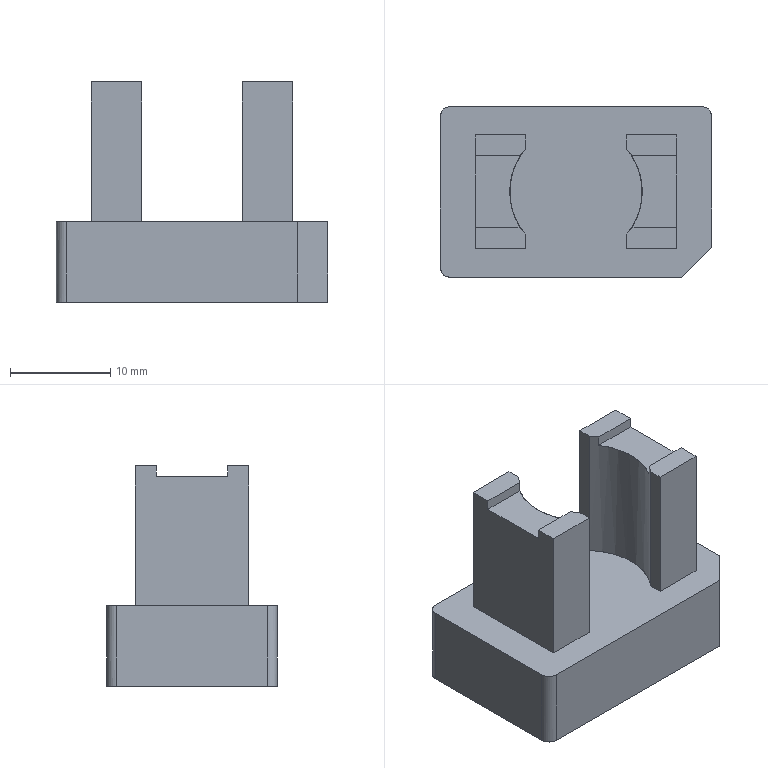NC program | PowerMill | posted with a generic post | part box 27 x 17 x 21.929 mm
Lines 15673 to 16510 of 116051:
N15770 M6
N15771 S8500 M03
N15772 G00 G90 X0.0 Y0.0
N15773 G43 Z11.799 H3
N15774
N15775 G05 P10000 R8
N15776 X-20.8023 Y3.3412
N15777 Z-0.0874
N15778 G01 Z-1.2874 F360.0
N15779 X-15.5273 Y3.3411 F600.0
N15780 X-15.5261 Y3.3395
N15781 X-15.5249 Y3.338
N15782 X-15.525 Y-3.3282
N15783 G02 X-18.0361 Y-5.1559 I-1.9207 J0.0001
N15784 G01 X-20.9298 Y-4.2214
N15785 G02 X-20.8022 Y-3.384 I0.1319 J0.4083
N15786 G01 X-15.5275 Y-3.3313
N15787 G03 X-15.4003 Y-3.0217 I-0.4694 J0.3737
N15788 G01 X-15.3797 Y-2.8304
N15789 X-15.3342 Y-2.5473
N15790 X-15.2729 Y-2.2643
N15791 X-15.1951 Y-1.9813
N15792 X-15.1005 Y-1.6982
N15793 X-14.9876 Y-1.4152
N15794 X-14.8701 Y-1.1609
N15795 X-14.703 Y-0.8491
N15796 X-14.5271 Y-0.5661
N15797 X-14.3643 Y-0.3376
N15798 G03 X-14.3658 Y0.3609 I-0.4886 J0.3482
N15799 G01 X-14.5133 Y0.5661
N15800 X-14.6912 Y0.8491
N15801 X-14.8701 Y1.1813
N15802 X-14.9789 Y1.4152
N15803 X-15.0929 Y1.6982
N15804 X-15.1888 Y1.9813
N15805 X-15.2677 Y2.2643
N15806 X-15.3301 Y2.5473
N15807 X-15.377 Y2.8304
N15808 X-15.3995 Y3.0326
N15809 G03 X-15.5273 Y3.3411 I-0.5963 J-0.0664
N15810 G00 Z5.0256
N15811 G01 X20.8023 Y-3.3986 F10000.0
N15812 G00 Z-0.0874
N15813 G01 Z-1.2874 F360.0
N15814 X15.5273 Y-3.3985 F600.0
N15815 X15.5261 Y-3.3969
N15816 X15.5249 Y-3.3952
N15817 X15.525 Y3.3953
N15818 G02 X18.0364 Y5.2243 I1.9217 J0.0
N15819 G01 X20.9293 Y4.2916
N15820 G02 X20.8022 Y3.454 I-0.1317 J-0.4085
N15821 G01 X15.5275 Y3.3986
N15822 G03 X15.4069 Y3.0994 I0.4758 J-0.3656
N15823 G01 X15.377 Y2.8304
N15824 X15.3301 Y2.5473
N15825 X15.2678 Y2.2643
N15826 X15.1888 Y1.9813
N15827 X15.0931 Y1.6982
N15828 X14.9789 Y1.4152
N15829 X14.8701 Y1.1813
N15830 X14.6912 Y0.8491
N15831 X14.5134 Y0.5661
N15832 X14.3659 Y0.3613
N15833 G03 X14.3642 Y-0.3375 I0.4869 J-0.3506
N15834 G01 X14.5271 Y-0.5661
N15835 X14.703 Y-0.8491
N15836 X14.8701 Y-1.1609
N15837 X14.9876 Y-1.4152
N15838 X15.1003 Y-1.6982
N15839 X15.1951 Y-1.9813
N15840 X15.2727 Y-2.2643
N15841 X15.3342 Y-2.5473
N15842 X15.38 Y-2.8304
N15843 X15.4086 Y-3.0992
N15844 G03 X15.5273 Y-3.3985 I0.5967 J0.0634
N15845 G00 Z3.9986
N15846 G01 X20.6038 Y7.7104 F10000.0
N15847 G00 Z0.9286
N15848 G01 Z-0.2714 F360.0
N15849 X15.427 Y6.6972 F600.0
N15850 X-15.4311 Y6.6736
N15851 X-15.4711 Y6.4252
N15852 X-15.4923 Y6.2723
N15853 X-15.5162 Y6.0043
N15854 X-15.5273 Y5.6906
N15855 X-15.5267 Y3.4776
N15856 X-15.52 Y3.2898
N15857 X-15.5076 Y3.1023
N15858 X-15.4759 Y2.8185
N15859 X-15.4264 Y2.5206
N15860 X-15.3586 Y2.2167
N15861 X15.3645 Y2.2402
N15862 X15.2701 Y1.9104
N15863 G02 X15.0251 Y1.278 I-4.8516 J1.5155
N15864 G01 X14.9676 Y1.1536
N15865 X14.9034 Y1.0326
N15866 G02 X14.6989 Y0.6739 I-2.9966 J1.4707
N15867 G01 X14.6427 Y0.5807
N15868 X14.5195 Y0.4007
N15869 X14.3907 Y0.2247
N15870 X14.215 Y0.0091
N15871 X14.4025 Y-0.2197
N15872 X14.5313 Y-0.3983
N15873 X14.6556 Y-0.5801
N15874 X14.7861 Y-0.7934
N15875 X14.8469 Y-0.9009
N15876 X14.903 Y-1.011
N15877 G02 X15.114 Y-1.4631 I-3.5225 J-1.9195
N15878 G01 X15.1758 Y-1.6152
N15879 X15.2821 Y-1.9253
N15880 X15.3637 Y-2.2167
N15881 X-15.3696 Y-2.2402
N15882 X-15.4323 Y-2.5298
N15883 X-15.4792 Y-2.8228
N15884 X-15.5097 Y-3.1073
N15885 X-15.5212 Y-3.2923
N15886 X-15.527 Y-3.4776
N15887 X-15.5273 Y-5.6942
N15888 X-15.5159 Y-6.0104
N15889 X-15.4846 Y-6.3385
N15890 X-15.4585 Y-6.5183
N15891 X-15.4267 Y-6.6972
N15892 X15.4311 Y-6.6736
N15893 G00 Z11.799
N15894 G05 P0
N15895 (---------------)
N15896 ( END TOOLPATH : 精公基准台01-平坦面平行-D10 )
N15897 (---------------)
N15898 ( START TOOLPATH : 精公基准台01-基准面偏置-D10 )
N15899 (---------------)
N15900 G00 X0.0 Y0.0 Z9.7986
N15901 G05 P10000 R8
N15902 X23.9651 Y-7.9718
N15903 Z-12.93
N15904 G01 Z-14.13 F360.0
N15905 X18.8237 Y-6.7923 F600.0
N15906 X15.4276 Y0.0
N15907 Y-5.3835
N15908 X15.4196 Y-5.9502
N15909 X15.3963 Y-6.2335
N15910 X15.3582 Y-6.5169
N15911 X15.3043 Y-6.8002
N15912 X15.2343 Y-7.0836
N15913 X15.1482 Y-7.3669
N15914 X15.0439 Y-7.6502
N15915 X14.9379 Y-7.8973
N15916 X14.7783 Y-8.2169
N15917 X14.6134 Y-8.5003
N15918 X14.4243 Y-8.7836
N15919 X14.1792 Y-9.1006
N15920 X13.9575 Y-9.3503
N15921 X13.8105 Y-9.4997
N15922 X13.5698 Y-9.7215
N15923 X13.3305 Y-9.917
N15924 X13.2468 Y-9.9801
N15925 X12.965 Y-10.1752
N15926 X12.6831 Y-10.345
N15927 X12.4194 Y-10.4837
N15928 X12.1194 Y-10.6198
N15929 X11.8376 Y-10.7282
N15930 X11.5557 Y-10.819
N15931 X11.2739 Y-10.8932
N15932 X10.992 Y-10.9513
N15933 X10.7102 Y-10.9939
N15934 X10.4283 Y-11.0213
N15935 X10.1465 Y-11.0339
N15936 X5.3551 Y-11.0348
N15937 X4.7914 Y-11.0312
N15938 X4.5096 Y-11.0136
N15939 X4.2277 Y-10.9812
N15940 X3.9459 Y-10.9332
N15941 X3.664 Y-10.8697
N15942 X3.3822 Y-10.7901
N15943 X3.1003 Y-10.6934
N15944 X2.8574 Y-10.5956
N15945 X2.5366 Y-10.4446
N15946 X2.2548 Y-10.2899
N15947 X1.9729 Y-10.1118
N15948 X1.7035 Y-9.917
N15949 X1.4092 Y-9.6732
N15950 X1.2429 Y-9.5189
N15951 X1.0765 Y-9.3503
N15952 X0.8455 Y-9.0896
N15953 X0.792 Y-9.0202
N15954 G03 X-0.792 I-0.792 J-0.6105
N15955 G01 X-0.8455 Y-9.0896
N15956 X-1.0765 Y-9.3503
N15957 X-1.2429 Y-9.5189
N15958 X-1.4092 Y-9.6732
N15959 X-1.7035 Y-9.917
N15960 X-1.9729 Y-10.1118
N15961 X-2.2548 Y-10.2899
N15962 X-2.5366 Y-10.4446
N15963 X-2.8574 Y-10.5956
N15964 X-3.1003 Y-10.6934
N15965 X-3.3822 Y-10.7901
N15966 X-3.664 Y-10.8697
N15967 X-3.9459 Y-10.9332
N15968 X-4.2277 Y-10.9812
N15969 X-4.5096 Y-11.0136
N15970 X-4.7914 Y-11.0312
N15971 X-5.3551 Y-11.0348
N15972 X-10.1465 Y-11.0339
N15973 X-10.4283 Y-11.0213
N15974 X-10.7102 Y-10.9939
N15975 X-10.992 Y-10.9513
N15976 X-11.2739 Y-10.8932
N15977 X-11.5557 Y-10.819
N15978 X-11.8376 Y-10.7282
N15979 X-12.1194 Y-10.6198
N15980 X-12.4194 Y-10.4837
N15981 X-12.6831 Y-10.345
N15982 X-12.965 Y-10.1752
N15983 X-13.2468 Y-9.9801
N15984 X-13.3305 Y-9.917
N15985 X-13.5705 Y-9.721
N15986 X-13.8105 Y-9.4997
N15987 X-13.9575 Y-9.3503
N15988 X-14.1787 Y-9.1013
N15989 X-14.4243 Y-8.7836
N15990 X-14.6135 Y-8.5003
N15991 X-14.7783 Y-8.2169
N15992 X-14.9379 Y-7.8973
N15993 X-15.0439 Y-7.6502
N15994 X-15.1478 Y-7.3669
N15995 X-15.2343 Y-7.0836
N15996 X-15.3042 Y-6.8002
N15997 X-15.3582 Y-6.5169
N15998 X-15.3964 Y-6.2335
N15999 X-15.4196 Y-5.9502
N16000 X-15.4276 Y-5.3835
N16001 Y5.3835
N16002 X-15.4196 Y5.9502
N16003 X-15.3964 Y6.2335
N16004 X-15.3582 Y6.5169
N16005 X-15.3042 Y6.8002
N16006 X-15.2343 Y7.0836
N16007 X-15.1478 Y7.3669
N16008 X-15.0439 Y7.6502
N16009 X-14.9379 Y7.8973
N16010 X-14.7783 Y8.2169
N16011 X-14.6135 Y8.5003
N16012 X-14.4243 Y8.7836
N16013 X-14.1793 Y9.1006
N16014 X-13.9575 Y9.3503
N16015 X-13.8105 Y9.4997
N16016 X-13.5698 Y9.7215
N16017 X-13.3305 Y9.917
N16018 X-13.2468 Y9.9801
N16019 X-12.965 Y10.1752
N16020 X-12.6831 Y10.345
N16021 X-12.4194 Y10.4837
N16022 X-12.1194 Y10.6198
N16023 X-11.8376 Y10.7284
N16024 X-11.5557 Y10.819
N16025 X-11.2739 Y10.8934
N16026 X-10.992 Y10.9513
N16027 X-10.7102 Y10.9938
N16028 X-10.4283 Y11.0213
N16029 X-10.1465 Y11.0338
N16030 X-5.3551 Y11.0348
N16031 X-4.7914 Y11.0312
N16032 X-4.5096 Y11.0138
N16033 X-4.2277 Y10.9812
N16034 X-3.9459 Y10.9333
N16035 X-3.664 Y10.8697
N16036 X-3.3822 Y10.7904
N16037 X-3.1003 Y10.6934
N16038 X-2.8582 Y10.5964
N16039 X-2.5366 Y10.4446
N16040 X-2.2548 Y10.2897
N16041 X-1.9729 Y10.1118
N16042 X-1.7035 Y9.917
N16043 X-1.4092 Y9.6732
N16044 X-1.2434 Y9.5193
N16045 X-1.0765 Y9.3503
N16046 X-0.8455 Y9.0896
N16047 X-0.792 Y9.0202
N16048 G03 X0.792 I0.792 J0.6105
N16049 G01 X0.8455 Y9.0896
N16050 X1.0765 Y9.3503
N16051 X1.2429 Y9.5188
N16052 X1.4092 Y9.6732
N16053 X1.7035 Y9.917
N16054 X1.9729 Y10.1118
N16055 X2.2548 Y10.2897
N16056 X2.5366 Y10.4446
N16057 X2.8574 Y10.5959
N16058 X3.1003 Y10.6934
N16059 X3.3822 Y10.7904
N16060 X3.664 Y10.8697
N16061 X3.9459 Y10.9333
N16062 X4.2277 Y10.9812
N16063 X4.5096 Y11.0138
N16064 X4.7914 Y11.0312
N16065 X5.3551 Y11.0348
N16066 X10.1465 Y11.0338
N16067 X10.4283 Y11.0213
N16068 X10.7102 Y10.9938
N16069 X10.992 Y10.9513
N16070 X11.2739 Y10.8934
N16071 X11.5557 Y10.819
N16072 X11.8376 Y10.7284
N16073 X12.1194 Y10.6198
N16074 X12.4194 Y10.4837
N16075 X12.6831 Y10.345
N16076 X12.965 Y10.1752
N16077 X13.2468 Y9.9801
N16078 X13.3305 Y9.917
N16079 X13.5698 Y9.7215
N16080 X13.8105 Y9.4997
N16081 X13.9575 Y9.3503
N16082 X14.1792 Y9.1006
N16083 X14.4243 Y8.7836
N16084 X14.6134 Y8.5003
N16085 X14.7783 Y8.2169
N16086 X14.9379 Y7.8973
N16087 X15.0439 Y7.6502
N16088 X15.1482 Y7.3669
N16089 X15.2343 Y7.0836
N16090 X15.3043 Y6.8002
N16091 X15.3582 Y6.5169
N16092 X15.3963 Y6.2335
N16093 X15.4196 Y5.9502
N16094 X15.4276 Y5.3835
N16095 Y0.0
N16096 G00 Z9.7986
N16097 G05 P0
N16098 (---------------)
N16099 ( END TOOLPATH : 精公基准台01-基准面偏置-D10 )
N16100 (---------------)
N16101 ( START TOOLPATH : 精公基准台01-基准台侧光-D10 )
N16102 (---------------)
N16103 G00 X0.0 Y0.0 Z9.7986
N16104 G05 P10000 R8
N16105 X18.4748 Y-14.7804
N16106 Z-20.83
N16107 G01 Z-22.03 F360.0
N16108 G03 X14.9391 Y-11.2451 I-1.7679 J1.7677 F600.0
N16109 G01 X14.1141 Y-12.0701
N16110 X14.1137 Y-12.0705
N16111 X14.1133 Y-12.0709
N16112 X13.9661 Y-12.2138
N16113 X13.9648 Y-12.2151
N16114 X13.9634 Y-12.2163
N16115 X13.7676 Y-12.3896
N16116 X13.7664 Y-12.3907
N16117 X13.7651 Y-12.3917
N16118 X13.6447 Y-12.4896
N16119 X13.6431 Y-12.4909
N16120 X13.6414 Y-12.4922
N16121 X13.3422 Y-12.7105
N16122 X13.3397 Y-12.7122
N16123 X13.3371 Y-12.7139
N16124 X13.0041 Y-12.9199
N16125 X13.0019 Y-12.9212
N16126 X12.9997 Y-12.9224
N16127 X12.7941 Y-13.0325
N16128 X12.7928 Y-13.0332
N16129 X12.7915 Y-13.0338
N16130 X12.681 Y-13.088
N16131 X12.6794 Y-13.0888
N16132 X12.6776 Y-13.0895
N16133 X12.3615 Y-13.2266
N16134 X12.3588 Y-13.2277
N16135 X12.3561 Y-13.2287
N16136 X11.9994 Y-13.3536
N16137 X11.9969 Y-13.3545
N16138 X11.9943 Y-13.3552
N16139 X11.7188 Y-13.4316
N16140 X11.7164 Y-13.4322
N16141 X11.714 Y-13.4328
N16142 X11.3979 Y-13.5
N16143 X11.3954 Y-13.5005
N16144 X11.3928 Y-13.5009
N16145 X11.0767 Y-13.5471
N16146 X11.0742 Y-13.5475
N16147 X11.0716 Y-13.5477
N16148 X10.7555 Y-13.5735
N16149 X10.753 Y-13.5737
N16150 X10.7505 Y-13.5738
N16151 X10.4344 Y-13.58
N16152 X10.4336
N16153 X10.4328
N16154 X-12.3297
N16155 X-12.33
N16156 X-12.3302
N16157 X-12.6464 Y-13.5779
N16158 X-12.6481 Y-13.5778
N16159 X-12.6498
N16160 X-12.9659 Y-13.5621
N16161 X-12.9681 Y-13.562
N16162 X-12.9702 Y-13.5618
N16163 X-13.2864 Y-13.5289
N16164 X-13.2885 Y-13.5287
N16165 X-13.2906 Y-13.5284
N16166 X-13.6068 Y-13.4783
N16167 X-13.6089 Y-13.478
N16168 X-13.611 Y-13.4776
N16169 X-13.9271 Y-13.4101
N16170 X-13.9292 Y-13.4096
N16171 X-13.9313 Y-13.4091
N16172 X-14.2475 Y-13.3234
N16173 X-14.2496 Y-13.3228
N16174 X-14.2518 Y-13.3221
N16175 X-14.5679 Y-13.217
N16176 X-14.57 Y-13.2163
N16177 X-14.572 Y-13.2156
N16178 X-14.8881 Y-13.0912
N16179 X-14.8896 Y-13.0906
N16180 X-14.8911 Y-13.09
N16181 X-15.0155 Y-13.0352
N16182 X-15.0167 Y-13.0347
N16183 X-15.0178 Y-13.0341
N16184 X-15.2095 Y-12.9423
N16185 X-15.2111 Y-12.9416
N16186 X-15.2127 Y-12.9407
N16187 X-15.5288 Y-12.7718
N16188 X-15.531 Y-12.7706
N16189 X-15.5332 Y-12.7693
N16190 X-15.8493 Y-12.5742
N16191 X-15.8514 Y-12.5729
N16192 X-15.8535 Y-12.5715
N16193 X-16.1697 Y-12.3476
N16194 X-16.1718 Y-12.346
N16195 X-16.1739 Y-12.3444
N16196 X-16.49 Y-12.0875
N16197 X-16.4922 Y-12.0857
N16198 X-16.4942 Y-12.0839
N16199 X-16.8104 Y-11.7879
N16200 X-16.8126 Y-11.7858
N16201 X-16.8147 Y-11.7836
N16202 X-17.1308 Y-11.4389
N16203 X-17.1327 Y-11.4368
N16204 X-17.1345 Y-11.4346
N16205 X-17.3886 Y-11.1149
N16206 X-17.3902 Y-11.1127
N16207 X-17.3918 Y-11.1105
N16208 X-17.6098 Y-10.7944
N16209 X-17.611 Y-10.7925
N16210 X-17.6122 Y-10.7906
N16211 X-17.7725 Y-10.5277
N16212 X-17.7737 Y-10.5256
N16213 X-17.7749 Y-10.5235
N16214 X-17.9701 Y-10.154
N16215 X-17.9712 Y-10.1519
N16216 X-17.9722 Y-10.1498
N16217 X-18.0931 Y-9.8838
N16218 X-18.094 Y-9.8817
N16219 X-18.0949 Y-9.8796
N16220 X-18.2369 Y-9.5133
N16221 X-18.2377 Y-9.511
N16222 X-18.2385 Y-9.5087
N16223 X-18.3396 Y-9.1926
N16224 X-18.3402 Y-9.1906
N16225 X-18.3408 Y-9.1886
N16226 X-18.4138 Y-8.9117
N16227 X-18.4143 Y-8.9095
N16228 X-18.4148 Y-8.9073
N16229 X-18.4875 Y-8.552
N16230 X-18.4879 Y-8.5499
N16231 X-18.4883 Y-8.5478
N16232 X-18.5357 Y-8.2317
N16233 X-18.536 Y-8.2294
N16234 X-18.5363 Y-8.2271
N16235 X-18.5653 Y-7.911
N16236 X-18.5655 Y-7.909
N16237 X-18.5656 Y-7.9071
N16238 X-18.5792 Y-7.5909
N16239 Y-7.5892
N16240 Y-7.5875
N16241 Y7.5875
N16242 Y7.5891
N16243 Y7.5907
N16244 X-18.5664 Y7.9069
N16245 X-18.5662 Y7.909
N16246 X-18.5661 Y7.9112
N16247 X-18.5362 Y8.2273
N16248 X-18.536 Y8.2294
N16249 X-18.5357 Y8.2315
N16250 X-18.489 Y8.5476
N16251 X-18.4887 Y8.5498
N16252 X-18.4883 Y8.5519
N16253 X-18.424 Y8.868
N16254 X-18.4236 Y8.8701
N16255 X-18.423 Y8.8722
N16256 X-18.3408 Y9.1884
N16257 X-18.3402 Y9.1905
N16258 X-18.3395 Y9.1926
N16259 X-18.2384 Y9.5087
N16260 X-18.2377 Y9.5108
N16261 X-18.2369 Y9.5129
N16262 X-18.1162 Y9.8291
N16263 X-18.1153 Y9.8312
N16264 X-18.1144 Y9.8334
N16265 X-17.9721 Y10.1495
N16266 X-17.9711 Y10.1516
N16267 X-17.9701 Y10.1537
N16268 X-17.8052 Y10.4698
N16269 X-17.804 Y10.4719
N16270 X-17.8028 Y10.4741
N16271 X-17.6126 Y10.7902
N16272 X-17.6115 Y10.792
N16273 X-17.6103 Y10.7938
N16274 X-17.4543 Y11.0244
N16275 X-17.4535 Y11.0255
N16276 X-17.4528 Y11.0265
N16277 X-17.3907 Y11.1121
N16278 X-17.3897 Y11.1134
N16279 X-17.3887 Y11.1148
N16280 X-17.1383 Y11.4309
N16281 X-17.1365 Y11.4331
N16282 X-17.1347 Y11.4351
N16283 X-16.8464 Y11.7513
N16284 X-16.8444 Y11.7534
N16285 X-16.8423 Y11.7555
N16286 X-16.508 Y12.0717
N16287 X-16.5059 Y12.0736
N16288 X-16.5036 Y12.0755
N16289 X-16.174 Y12.3443
N16290 X-16.1718 Y12.346
N16291 X-16.1695 Y12.3477
N16292 X-15.8534 Y12.5707
N16293 X-15.8518 Y12.5719
N16294 X-15.8501 Y12.573
N16295 X-15.6282 Y12.7134
N16296 X-15.6271 Y12.7141
N16297 X-15.626 Y12.7148
N16298 X-15.5317 Y12.7702
N16299 X-15.5303 Y12.771
N16300 X-15.5289 Y12.7718
N16301 X-15.2128 Y12.9412
N16302 X-15.2107 Y12.9423
N16303 X-15.2085 Y12.9433
N16304 X-14.8924 Y13.0894
N16305 X-14.8903 Y13.0903
N16306 X-14.8882 Y13.0912
N16307 X-14.5721 Y13.216
N16308 X-14.57 Y13.2168
N16309 X-14.5678 Y13.2175
N16310 X-14.2517 Y13.3222
N16311 X-14.2496 Y13.3228
N16312 X-14.2475 Y13.3234
N16313 X-13.9313 Y13.4091
N16314 X-13.9292 Y13.4096
N16315 X-13.927 Y13.4101
N16316 X-13.6109 Y13.4772
N16317 X-13.6089 Y13.4776
N16318 X-13.6069 Y13.478
N16319 X-13.2907 Y13.5283
N16320 X-13.2885 Y13.5287
N16321 X-13.2863 Y13.5289
N16322 X-12.9701 Y13.5614
N16323 X-12.9681 Y13.5615
N16324 X-12.966 Y13.5617
N16325 X-12.6499 Y13.5778
N16326 X-12.6481
N16327 X-12.6464 Y13.5779
N16328 X-12.3302 Y13.58
N16329 X-12.33
N16330 X-12.3297
N16331 X0.0
N16332 X12.3297
N16333 X12.33
N16334 X12.3302
N16335 X12.6464 Y13.5779
N16336 X12.6481 Y13.5778
N16337 X12.6498
N16338 X12.9659 Y13.5621
N16339 X12.9681 Y13.562
N16340 X12.9702 Y13.5618
N16341 X13.2864 Y13.5289
N16342 X13.2885 Y13.5287
N16343 X13.2906 Y13.5284
N16344 X13.6068 Y13.4783
N16345 X13.6089 Y13.478
N16346 X13.611 Y13.4776
N16347 X13.9271 Y13.4101
N16348 X13.9292 Y13.4096
N16349 X13.9313 Y13.4091
N16350 X14.2475 Y13.3234
N16351 X14.2496 Y13.3228
N16352 X14.2518 Y13.3221
N16353 X14.5679 Y13.217
N16354 X14.57 Y13.2163
N16355 X14.572 Y13.2156
N16356 X14.8881 Y13.0912
N16357 X14.8896 Y13.0906
N16358 X14.8911 Y13.09
N16359 X15.0155 Y13.0352
N16360 X15.0167 Y13.0347
N16361 X15.0178 Y13.0341
N16362 X15.2095 Y12.9423
N16363 X15.2111 Y12.9416
N16364 X15.2127 Y12.9407
N16365 X15.5288 Y12.7718
N16366 X15.531 Y12.7706
N16367 X15.5332 Y12.7693
N16368 X15.8493 Y12.5742
N16369 X15.8514 Y12.5729
N16370 X15.8535 Y12.5715
N16371 X16.1697 Y12.3476
N16372 X16.1718 Y12.346
N16373 X16.1739 Y12.3444
N16374 X16.49 Y12.0875
N16375 X16.4922 Y12.0857
N16376 X16.4942 Y12.0839
N16377 X16.8104 Y11.7879
N16378 X16.8126 Y11.7858
N16379 X16.8147 Y11.7836
N16380 X17.1308 Y11.4389
N16381 X17.1327 Y11.4368
N16382 X17.1345 Y11.4346
N16383 X17.3886 Y11.1149
N16384 X17.3902 Y11.1127
N16385 X17.3918 Y11.1105
N16386 X17.6098 Y10.7944
N16387 X17.611 Y10.7925
N16388 X17.6122 Y10.7906
N16389 X17.7725 Y10.5277
N16390 X17.7737 Y10.5256
N16391 X17.7749 Y10.5235
N16392 X17.9701 Y10.154
N16393 X17.9712 Y10.1519
N16394 X17.9722 Y10.1498
N16395 X18.0931 Y9.8838
N16396 X18.094 Y9.8817
N16397 X18.0949 Y9.8796
N16398 X18.2369 Y9.5133
N16399 X18.2377 Y9.511
N16400 X18.2385 Y9.5087
N16401 X18.3396 Y9.1926
N16402 X18.3402 Y9.1906
N16403 X18.3408 Y9.1886
N16404 X18.4138 Y8.9117
N16405 X18.4143 Y8.9095
N16406 X18.4148 Y8.9073
N16407 X18.4875 Y8.552
N16408 X18.4879 Y8.5499
N16409 X18.4883 Y8.5478
N16410 X18.5357 Y8.2317
N16411 X18.536 Y8.2294
N16412 X18.5363 Y8.2271
N16413 X18.5653 Y7.911
N16414 X18.5655 Y7.909
N16415 X18.5656 Y7.9071
N16416 X18.5792 Y7.5909
N16417 Y7.5892
N16418 Y7.5875
N16419 X18.58 Y-5.3745
N16420 Y-5.3749
N16421 Y-5.3754
N16422 X18.5764 Y-5.6915
N16423 X18.5763 Y-5.6939
N16424 X18.5762 Y-5.6962
N16425 X18.5541 Y-6.0124
N16426 X18.5538 Y-6.0149
N16427 X18.5535 Y-6.0174
N16428 X18.5111 Y-6.3336
N16429 X18.5107 Y-6.3361
N16430 X18.5103 Y-6.3386
N16431 X18.447 Y-6.6548
N16432 X18.4466 Y-6.6565
N16433 X18.4462 Y-6.6583
N16434 X18.4141 Y-6.7876
N16435 X18.4138 Y-6.7889
N16436 X18.4134 Y-6.7902
N16437 X18.3605 Y-6.977
N16438 X18.3599 Y-6.979
N16439 X18.3593 Y-6.981
N16440 X18.2514 Y-7.2972
N16441 X18.2505 Y-7.2997
N16442 X18.2495 Y-7.3022
N16443 X18.1172 Y-7.6184
N16444 X18.1161 Y-7.6209
N16445 X18.1149 Y-7.6234
N16446 X17.9558 Y-7.9396
N16447 X17.9545 Y-7.9421
N16448 X17.9531 Y-7.9446
N16449 X17.7729 Y-8.2474
N16450 X17.7713 Y-8.25
N16451 X17.7696 Y-8.2525
N16452 X17.5383 Y-8.5819
N16453 X17.537 Y-8.5837
N16454 X17.5357 Y-8.5854
N16455 X17.4509 Y-8.6932
N16456 X17.4499 Y-8.6945
N16457 X17.4488 Y-8.6958
N16458 X17.2707 Y-8.9041
N16459 X17.2695 Y-8.9055
N16460 X17.2682 Y-8.9069
N16461 X17.1301 Y-9.0537
N16462 X17.1293 Y-9.0545
N16463 X17.1284 Y-9.0554
N16464 X14.9391 Y-11.2451
N16465 G03 X18.4748 Y-14.7804 I1.7678 J-1.7676
N16466 G01 X18.4233 Y-14.7187
N16467 G03 X14.8875 Y-11.1834 I-1.7679 J1.7676
N16468 G01 X14.0575 Y-12.0135
N16469 X13.9104 Y-12.1564
N16470 X13.7146 Y-12.3297
N16471 X13.5943 Y-12.4275
N16472 X13.295 Y-12.6458
N16473 X12.962 Y-12.8519
N16474 X12.7563 Y-12.962
N16475 X12.6458 Y-13.0161
N16476 X12.3297 Y-13.1532
N16477 X11.973 Y-13.2781
N16478 X11.6974 Y-13.3545
N16479 X11.3812 Y-13.4217
N16480 X11.0651 Y-13.468
N16481 X10.749 Y-13.4938
N16482 X10.4328 Y-13.5
N16483 X-12.3297
N16484 X-12.6458 Y-13.4979
N16485 X-12.962 Y-13.4822
N16486 X-13.2781 Y-13.4493
N16487 X-13.5943 Y-13.3993
N16488 X-13.9104 Y-13.3319
N16489 X-14.2266 Y-13.2462
N16490 X-14.5427 Y-13.1411
N16491 X-14.8588 Y-13.0168
N16492 X-14.9833 Y-12.962
N16493 X-15.175 Y-12.8702
N16494 X-15.4911 Y-12.7013
N16495 X-15.8073 Y-12.5062
N16496 X-16.1234 Y-12.2823
N16497 X-16.4396 Y-12.0254
N16498 X-16.7557 Y-11.7295
N16499 X-17.0719 Y-11.3849
N16500 X-17.3259 Y-11.0651
N16501 X-17.5439 Y-10.749
N16502 X-17.7042 Y-10.4861
N16503 X-17.8993 Y-10.1167
N16504 X-18.0203 Y-9.8507
N16505 X-18.1623 Y-9.4844
N16506 X-18.2634 Y-9.1682
N16507 X-18.3364 Y-8.8913
N16508 X-18.4091 Y-8.5359
N16509 X-18.4566 Y-8.2198
N16510 X-18.4856 Y-7.9036
N16511 X-18.4992 Y-7.5875
N16512 X-18.5 Y-7.2714
N16513 Y7.2714
N16514 X-18.4992 Y7.5875
N16515 X-18.4864 Y7.9036
N16516 X-18.4566 Y8.2198
N16517 X-18.4099 Y8.5359
N16518 X-18.3456 Y8.8521
N16519 X-18.2633 Y9.1682
N16520 X-18.1622 Y9.4844
N16521 X-18.0415 Y9.8005
N16522 X-17.8992 Y10.1167
N16523 X-17.7343 Y10.4328
N16524 X-17.544 Y10.749
N16525 X-17.388 Y10.9796
N16526 X-17.3259 Y11.0651
N16527 X-17.0756 Y11.3812
N16528 X-16.7873 Y11.6974
N16529 X-16.4531 Y12.0135
N16530 X-16.1234 Y12.2823
N16531 X-15.8073 Y12.5054
N16532 X-15.5854 Y12.6458
N16533 X-15.4911 Y12.7013
N16534 X-15.175 Y12.8707
N16535 X-14.8588 Y13.0168
N16536 X-14.5427 Y13.1416
N16537 X-14.2266 Y13.2462
N16538 X-13.9104 Y13.3318
N16539 X-13.5943 Y13.399
N16540 X-13.2781 Y13.4493
N16541 X-12.962 Y13.4818
N16542 X-12.6458 Y13.4979
N16543 X-12.3297 Y13.5
N16544 X0.0
N16545 X12.3297
N16546 X12.6458 Y13.4979
N16547 X12.962 Y13.4822
N16548 X13.2781 Y13.4493
N16549 X13.5943 Y13.3993
N16550 X13.9104 Y13.3319
N16551 X14.2266 Y13.2462
N16552 X14.5427 Y13.1411
N16553 X14.8588 Y13.0168
N16554 X14.9833 Y12.962
N16555 X15.175 Y12.8702
N16556 X15.4911 Y12.7013
N16557 X15.8073 Y12.5062
N16558 X16.1234 Y12.2823
N16559 X16.4396 Y12.0254
N16560 X16.7557 Y11.7295
N16561 X17.0719 Y11.3849
N16562 X17.3259 Y11.0651
N16563 X17.5439 Y10.749
N16564 X17.7042 Y10.4861
N16565 X17.8993 Y10.1167
N16566 X18.0203 Y9.8507
N16567 X18.1623 Y9.4844
N16568 X18.2634 Y9.1682
N16569 X18.3364 Y8.8913
N16570 X18.4091 Y8.5359
N16571 X18.4566 Y8.2198
N16572 X18.4856 Y7.9036
N16573 X18.4992 Y7.5875
N16574 X18.5 Y7.2714
N16575 Y-5.3745
N16576 X18.4964 Y-5.6906
N16577 X18.4743 Y-6.0068
N16578 X18.4318 Y-6.3229
N16579 X18.3685 Y-6.6391
N16580 X18.3364 Y-6.7684
N16581 X18.2836 Y-6.9552
N16582 X18.1757 Y-7.2714
N16583 X18.0434 Y-7.5875
N16584 X17.8844 Y-7.9036
N16585 X17.7042 Y-8.2065
N16586 X17.4728 Y-8.5359
N16587 X17.388 Y-8.6438
N16588 X17.2099 Y-8.8521
N16589 X17.0719 Y-8.9988
N16590 X14.8875 Y-11.1834
N16591 G03 X18.4233 Y-14.7187 I1.7679 J-1.7677
N16592 G00 Z9.7986
N16593 G05 P0
N16594 (---------------)
N16595 ( END TOOLPATH : 精公基准台01-基准台侧光-D10 )
N16596 (---------------)
N16597
N16598 M05
N16599 G53 Z0.0
N16600 (---------------)
N16601 ( START TOOLPATH : 精公精光01-等高-D4 )
N16602 (---------------)
N16603 ( TOOL NO.    :14 )
N16604 ( TOOL TYPE   : ENDMILL)
N16605 ( TOOL ID     : D4_1_1)
N16606 ( TOOL DIA    : 4.0 LENGTH 69.08)
N16607 T14